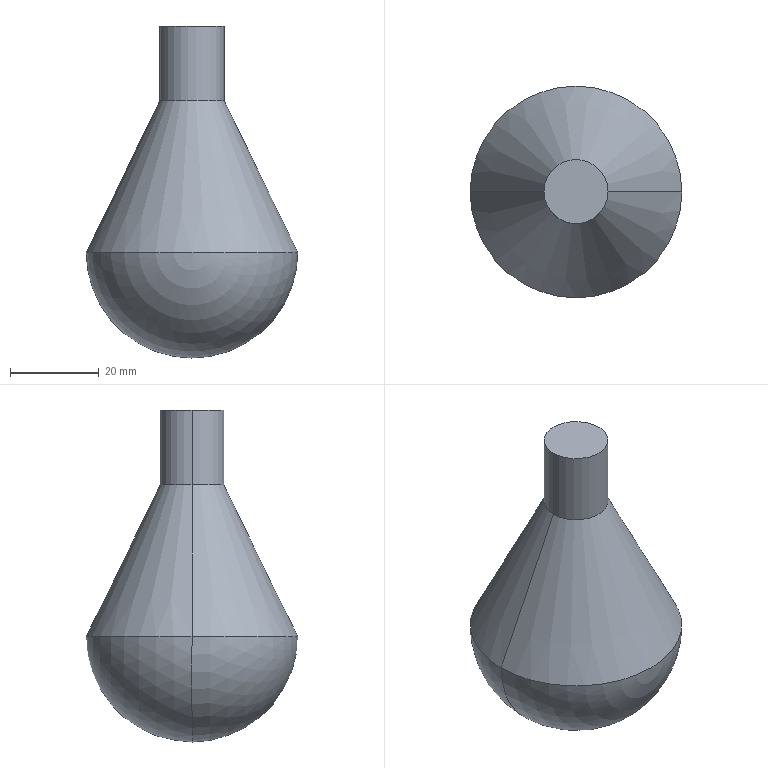Part | SolidWorks | features Revolution 1 | 1 solid | 7 faces | box 47.821 x 47.821 x 75.022 mm | volume 59967 mm3 | sphere 2 | cone 2 | cylinder 2 | plane 1 | commonest cylinder face diameters 14.48 x2
STEP:
#1=CARTESIAN_POINT('',(0.,0.,-75.022));
#2=VERTEX_POINT('',#1);
#3=CARTESIAN_POINT('',(23.91,0.,-51.112));
#4=VERTEX_POINT('',#3);
#5=CARTESIAN_POINT('',(0.,0.,-51.112));
#6=DIRECTION('',(0.,-1.,0.));
#7=DIRECTION('',(0.,0.,-1.));
#8=AXIS2_PLACEMENT_3D('',#5,#6,#7);
#9=CIRCLE('',#8,23.91);
#10=EDGE_CURVE('',#2,#4,#9,.T.);
#11=ORIENTED_EDGE('',*,*,#10,.F.);
#12=CARTESIAN_POINT('',(-23.91,0.,-51.112));
#13=VERTEX_POINT('',#12);
#14=CARTESIAN_POINT('',(0.,0.,-51.112));
#15=DIRECTION('',(0.,1.,0.));
#16=DIRECTION('',(-1.,0.,0.));
#17=AXIS2_PLACEMENT_3D('',#14,#15,#16);
#18=CIRCLE('',#17,23.91);
#19=EDGE_CURVE('',#2,#13,#18,.T.);
#20=ORIENTED_EDGE('',*,*,#19,.T.);
#21=CARTESIAN_POINT('',(0.,0.,-51.112));
#22=DIRECTION('',(0.,0.,1.));
#23=DIRECTION('',(1.,0.,0.));
#24=AXIS2_PLACEMENT_3D('',#21,#22,#23);
#25=CIRCLE('',#24,23.91);
#26=EDGE_CURVE('',#4,#13,#25,.T.);
#27=ORIENTED_EDGE('',*,*,#26,.F.);
#28=EDGE_LOOP('',(#11,#20,#27));
#29=FACE_OUTER_BOUND('',#28,.T.);
#30=CARTESIAN_POINT('',(0.,0.,-51.112));
#31=DIRECTION('',(0.,1.,0.));
#32=DIRECTION('',(1.,0.,0.));
#33=AXIS2_PLACEMENT_3D('',#30,#31,#32);
#34=SPHERICAL_SURFACE('',#33,23.91);
#35=ADVANCED_FACE('',(#29),#34,.T.);
#36=CARTESIAN_POINT('',(7.24,0.,-16.912));
#37=VERTEX_POINT('',#36);
#38=CARTESIAN_POINT('',(-7.24,0.,-16.912));
#39=VERTEX_POINT('',#38);
#40=CARTESIAN_POINT('',(0.,0.,-16.912));
#41=DIRECTION('',(0.,0.,1.));
#42=DIRECTION('',(1.,0.,0.));
#43=AXIS2_PLACEMENT_3D('',#40,#41,#42);
#44=CIRCLE('',#43,7.24);
#45=EDGE_CURVE('',#37,#39,#44,.T.);
#46=ORIENTED_EDGE('',*,*,#45,.F.);
#47=CARTESIAN_POINT('',(7.24,0.,-16.912));
#48=DIRECTION('',(0.4382,0.,-0.8989));
#49=VECTOR('',#48,1000.);
#50=LINE('',#47,#49);
#51=EDGE_CURVE('',#37,#4,#50,.T.);
#52=ORIENTED_EDGE('',*,*,#51,.T.);
#53=ORIENTED_EDGE('',*,*,#26,.T.);
#54=CARTESIAN_POINT('',(-7.24,0.,-16.912));
#55=DIRECTION('',(-0.4382,0.,-0.8989));
#56=VECTOR('',#55,1000.);
#57=LINE('',#54,#56);
#58=EDGE_CURVE('',#39,#13,#57,.T.);
#59=ORIENTED_EDGE('',*,*,#58,.F.);
#60=EDGE_LOOP('',(#46,#52,#53,#59));
#61=FACE_OUTER_BOUND('',#60,.T.);
#62=CARTESIAN_POINT('',(0.,0.,-16.912));
#63=DIRECTION('',(0.,0.,-1.));
#64=DIRECTION('',(-1.,0.,0.));
#65=AXIS2_PLACEMENT_3D('',#62,#63,#64);
#66=CONICAL_SURFACE('',#65,7.24,0.4536);
#67=ADVANCED_FACE('',(#61),#66,.T.);
#68=ORIENTED_EDGE('',*,*,#45,.T.);
#69=CARTESIAN_POINT('',(-7.24,0.,0.));
#70=VERTEX_POINT('',#69);
#71=CARTESIAN_POINT('',(-7.24,0.,-51.112));
#72=DIRECTION('',(0.,0.,1.));
#73=VECTOR('',#72,1000.);
#74=LINE('',#71,#73);
#75=EDGE_CURVE('',#39,#70,#74,.T.);
#76=ORIENTED_EDGE('',*,*,#75,.T.);
#77=CARTESIAN_POINT('',(7.24,0.,0.));
#78=VERTEX_POINT('',#77);
#79=CARTESIAN_POINT('',(0.,0.,0.));
#80=DIRECTION('',(0.,0.,1.));
#81=DIRECTION('',(1.,0.,0.));
#82=AXIS2_PLACEMENT_3D('',#79,#80,#81);
#83=CIRCLE('',#82,7.24);
#84=EDGE_CURVE('',#78,#70,#83,.T.);
#85=ORIENTED_EDGE('',*,*,#84,.F.);
#86=CARTESIAN_POINT('',(7.24,0.,-51.112));
#87=DIRECTION('',(0.,0.,1.));
#88=VECTOR('',#87,1000.);
#89=LINE('',#86,#88);
#90=EDGE_CURVE('',#37,#78,#89,.T.);
#91=ORIENTED_EDGE('',*,*,#90,.F.);
#92=EDGE_LOOP('',(#68,#76,#85,#91));
#93=FACE_OUTER_BOUND('',#92,.T.);
#94=CARTESIAN_POINT('',(0.,0.,-51.112));
#95=DIRECTION('',(0.,0.,1.));
#96=DIRECTION('',(1.,0.,0.));
#97=AXIS2_PLACEMENT_3D('',#94,#95,#96);
#98=CYLINDRICAL_SURFACE('',#97,7.24);
#99=ADVANCED_FACE('',(#93),#98,.T.);
#100=ORIENTED_EDGE('',*,*,#84,.T.);
#101=CARTESIAN_POINT('',(0.,0.,0.));
#102=DIRECTION('',(0.,0.,1.));
#103=DIRECTION('',(1.,0.,0.));
#104=AXIS2_PLACEMENT_3D('',#101,#102,#103);
#105=CIRCLE('',#104,7.24);
#106=EDGE_CURVE('',#70,#78,#105,.T.);
#107=ORIENTED_EDGE('',*,*,#106,.T.);
#108=EDGE_LOOP('',(#100,#107));
#109=FACE_OUTER_BOUND('',#108,.T.);
#110=CARTESIAN_POINT('',(0.,0.,0.));
#111=DIRECTION('',(0.,0.,1.));
#112=DIRECTION('',(1.,0.,0.));
#113=AXIS2_PLACEMENT_3D('',#110,#111,#112);
#114=PLANE('',#113);
#115=ADVANCED_FACE('',(#109),#114,.T.);
#116=ORIENTED_EDGE('',*,*,#75,.F.);
#117=CARTESIAN_POINT('',(0.,0.,-16.912));
#118=DIRECTION('',(0.,0.,1.));
#119=DIRECTION('',(1.,0.,0.));
#120=AXIS2_PLACEMENT_3D('',#117,#118,#119);
#121=CIRCLE('',#120,7.24);
#122=EDGE_CURVE('',#39,#37,#121,.T.);
#123=ORIENTED_EDGE('',*,*,#122,.T.);
#124=ORIENTED_EDGE('',*,*,#90,.T.);
#125=ORIENTED_EDGE('',*,*,#106,.F.);
#126=EDGE_LOOP('',(#116,#123,#124,#125));
#127=FACE_OUTER_BOUND('',#126,.T.);
#128=CARTESIAN_POINT('',(0.,0.,-51.112));
#129=DIRECTION('',(0.,0.,1.));
#130=DIRECTION('',(1.,0.,0.));
#131=AXIS2_PLACEMENT_3D('',#128,#129,#130);
#132=CYLINDRICAL_SURFACE('',#131,7.24);
#133=ADVANCED_FACE('',(#127),#132,.T.);
#134=ORIENTED_EDGE('',*,*,#51,.F.);
#135=ORIENTED_EDGE('',*,*,#122,.F.);
#136=ORIENTED_EDGE('',*,*,#58,.T.);
#137=CARTESIAN_POINT('',(0.,0.,-51.112));
#138=DIRECTION('',(0.,0.,1.));
#139=DIRECTION('',(1.,0.,0.));
#140=AXIS2_PLACEMENT_3D('',#137,#138,#139);
#141=CIRCLE('',#140,23.91);
#142=EDGE_CURVE('',#13,#4,#141,.T.);
#143=ORIENTED_EDGE('',*,*,#142,.T.);
#144=EDGE_LOOP('',(#134,#135,#136,#143));
#145=FACE_OUTER_BOUND('',#144,.T.);
#146=CARTESIAN_POINT('',(0.,0.,-16.912));
#147=DIRECTION('',(0.,0.,-1.));
#148=DIRECTION('',(-1.,0.,0.));
#149=AXIS2_PLACEMENT_3D('',#146,#147,#148);
#150=CONICAL_SURFACE('',#149,7.24,0.4536);
#151=ADVANCED_FACE('',(#145),#150,.T.);
#152=ORIENTED_EDGE('',*,*,#19,.F.);
#153=ORIENTED_EDGE('',*,*,#10,.T.);
#154=ORIENTED_EDGE('',*,*,#142,.F.);
#155=EDGE_LOOP('',(#152,#153,#154));
#156=FACE_OUTER_BOUND('',#155,.T.);
#157=CARTESIAN_POINT('',(0.,0.,-51.112));
#158=DIRECTION('',(0.,1.,0.));
#159=DIRECTION('',(1.,0.,0.));
#160=AXIS2_PLACEMENT_3D('',#157,#158,#159);
#161=SPHERICAL_SURFACE('',#160,23.91);
#162=ADVANCED_FACE('',(#156),#161,.T.);
#163=CLOSED_SHELL('',(#35,#67,#99,#115,#133,#151,#162));
#164=MANIFOLD_SOLID_BREP('',#163);
#165=CARTESIAN_POINT('',(0.,0.,0.));
#166=DIRECTION('',(0.,0.,1.));
#167=DIRECTION('',(1.,0.,0.));
#168=AXIS2_PLACEMENT_3D('',#165,#166,#167);
#169=(LENGTH_UNIT()NAMED_UNIT(*)SI_UNIT(.MILLI.,.METRE.));
#170=UNCERTAINTY_MEASURE_WITH_UNIT(LENGTH_MEASURE(0.00001),#169,'','');
#171=(NAMED_UNIT(*)PLANE_ANGLE_UNIT()SI_UNIT($,.RADIAN.));
#172=(NAMED_UNIT(*)SI_UNIT($,.STERADIAN.)SOLID_ANGLE_UNIT());
#173=(GEOMETRIC_REPRESENTATION_CONTEXT(3)GLOBAL_UNCERTAINTY_ASSIGNED_CONTEXT((#170))GLOBAL_UNIT_ASSIGNED_CONTEXT((#169,#171,#172))REPRESENTATION_CONTEXT('',''));
#174=ADVANCED_BREP_SHAPE_REPRESENTATION('',(#164,#168),#173);